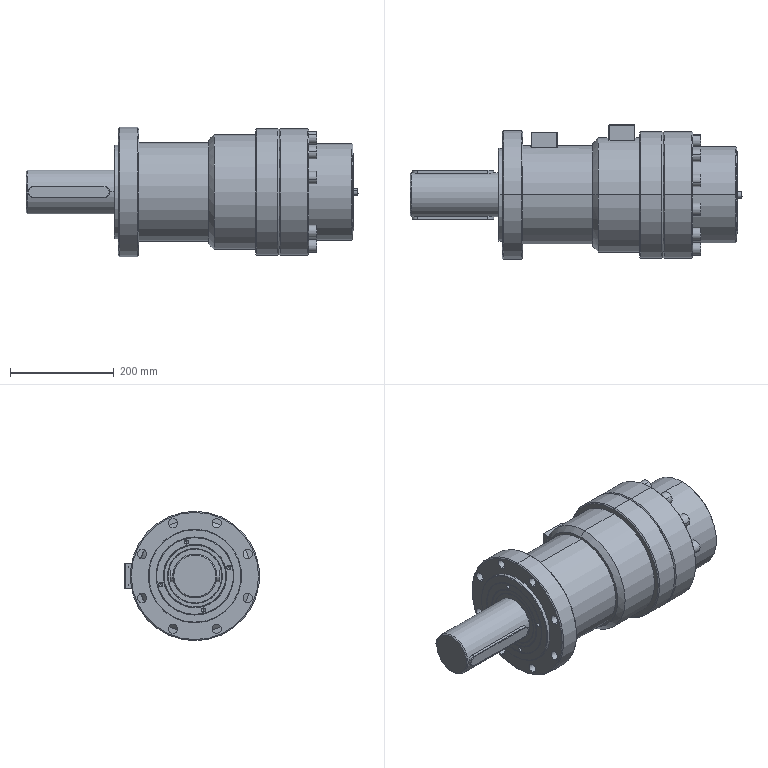Part | SolidWorks | features InContextFeatHolder 12, ReferencePattern 9, CompositeCurve 5, HoleSeries 3, AEMSimFeature 1, Cut 1, LocalCirPattern 1 | 64 solids | 3784 faces | volume 15807890 mm3 | plane 1289 | cylinder 937 | spline 582 | torus 508 | cone 468 | commonest cylinder face diameters 7.5 x232 0.75 x116 16 x44 110 x36 104.5 x32 14 x24